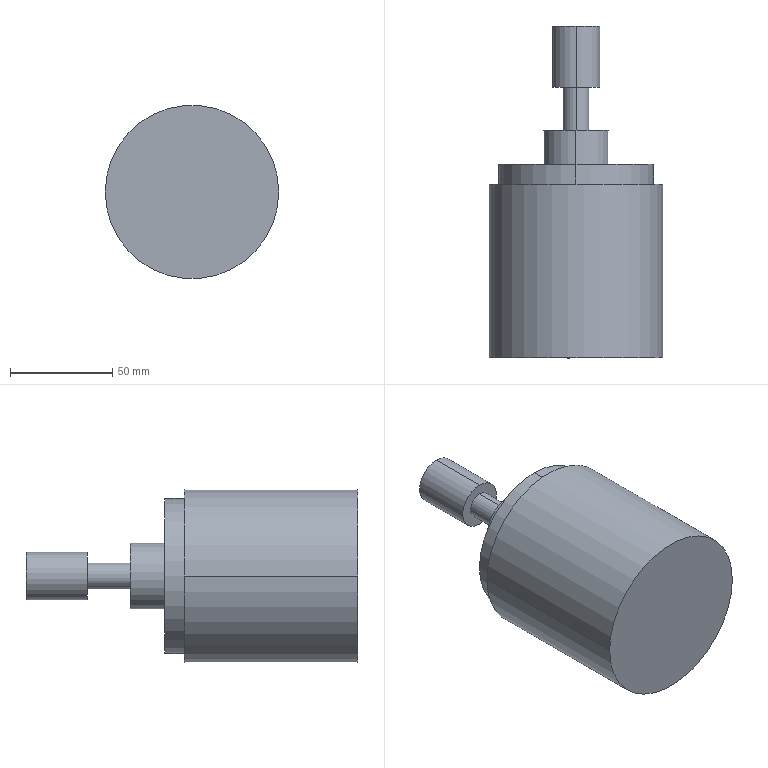Part | SolidWorks | features BaseBody 1 | 1 solid | 22 faces | box 85 x 162.58 x 85 mm | volume 554074 mm3 | cylinder 14 | plane 8 | commonest cylinder face diameters 12.708 x2 23.4 x2 32 x2 34 x2 45 x2 76 x2
STEP:
#1=CARTESIAN_POINT('',(2032.417,122.35,800.897));
#2=VERTEX_POINT('',#1);
#3=CARTESIAN_POINT('',(2032.417,122.35,876.897));
#4=VERTEX_POINT('',#3);
#5=CARTESIAN_POINT('',(2032.417,122.35,838.897));
#6=DIRECTION('',(0.,-1.,0.));
#7=DIRECTION('',(0.,0.,-1.));
#8=AXIS2_PLACEMENT_3D('',#5,#6,#7);
#9=CIRCLE('',#8,38.);
#10=EDGE_CURVE('',#2,#4,#9,.T.);
#11=ORIENTED_EDGE('',*,*,#10,.T.);
#12=CARTESIAN_POINT('',(2032.417,112.6,876.897));
#13=VERTEX_POINT('',#12);
#14=CARTESIAN_POINT('',(2032.417,122.35,876.897));
#15=DIRECTION('',(0.,-1.,0.));
#16=VECTOR('',#15,1000.);
#17=LINE('',#14,#16);
#18=EDGE_CURVE('',#4,#13,#17,.T.);
#19=ORIENTED_EDGE('',*,*,#18,.T.);
#20=CARTESIAN_POINT('',(2032.417,112.6,800.897));
#21=VERTEX_POINT('',#20);
#22=CARTESIAN_POINT('',(2032.417,112.6,838.897));
#23=DIRECTION('',(0.,1.,0.));
#24=DIRECTION('',(0.,0.,-1.));
#25=AXIS2_PLACEMENT_3D('',#22,#23,#24);
#26=CIRCLE('',#25,38.);
#27=EDGE_CURVE('',#13,#21,#26,.T.);
#28=ORIENTED_EDGE('',*,*,#27,.T.);
#29=CARTESIAN_POINT('',(2032.417,122.35,800.897));
#30=DIRECTION('',(0.,-1.,0.));
#31=VECTOR('',#30,1000.);
#32=LINE('',#29,#31);
#33=EDGE_CURVE('',#2,#21,#32,.T.);
#34=ORIENTED_EDGE('',*,*,#33,.F.);
#35=EDGE_LOOP('',(#11,#19,#28,#34));
#36=FACE_OUTER_BOUND('',#35,.T.);
#37=CARTESIAN_POINT('',(2032.417,122.35,838.897));
#38=DIRECTION('',(0.,-1.,0.));
#39=DIRECTION('',(0.,0.,-1.));
#40=AXIS2_PLACEMENT_3D('',#37,#38,#39);
#41=CYLINDRICAL_SURFACE('',#40,38.);
#42=ADVANCED_FACE('',(#36),#41,.T.);
#43=CARTESIAN_POINT('',(2074.917,112.6,838.897));
#44=VERTEX_POINT('',#43);
#45=CARTESIAN_POINT('',(1989.917,112.6,838.897));
#46=VERTEX_POINT('',#45);
#47=CARTESIAN_POINT('',(2032.417,112.6,838.897));
#48=DIRECTION('',(0.,-1.,0.));
#49=DIRECTION('',(0.,0.,1.));
#50=AXIS2_PLACEMENT_3D('',#47,#48,#49);
#51=CIRCLE('',#50,42.5);
#52=EDGE_CURVE('',#44,#46,#51,.T.);
#53=ORIENTED_EDGE('',*,*,#52,.T.);
#54=CARTESIAN_POINT('',(1989.917,27.6,838.897));
#55=VERTEX_POINT('',#54);
#56=CARTESIAN_POINT('',(1989.917,112.6,838.897));
#57=DIRECTION('',(0.,-1.,0.));
#58=VECTOR('',#57,1000.);
#59=LINE('',#56,#58);
#60=EDGE_CURVE('',#46,#55,#59,.T.);
#61=ORIENTED_EDGE('',*,*,#60,.T.);
#62=CARTESIAN_POINT('',(2074.917,27.6,838.897));
#63=VERTEX_POINT('',#62);
#64=CARTESIAN_POINT('',(2032.417,27.6,838.897));
#65=DIRECTION('',(0.,-1.,0.));
#66=DIRECTION('',(0.,0.,1.));
#67=AXIS2_PLACEMENT_3D('',#64,#65,#66);
#68=CIRCLE('',#67,42.5);
#69=EDGE_CURVE('',#63,#55,#68,.T.);
#70=ORIENTED_EDGE('',*,*,#69,.F.);
#71=CARTESIAN_POINT('',(2074.917,112.6,838.897));
#72=DIRECTION('',(0.,-1.,0.));
#73=VECTOR('',#72,1000.);
#74=LINE('',#71,#73);
#75=EDGE_CURVE('',#44,#63,#74,.T.);
#76=ORIENTED_EDGE('',*,*,#75,.F.);
#77=EDGE_LOOP('',(#53,#61,#70,#76));
#78=FACE_OUTER_BOUND('',#77,.T.);
#79=CARTESIAN_POINT('',(2032.417,112.6,838.897));
#80=DIRECTION('',(0.,-1.,0.));
#81=DIRECTION('',(1.,0.,0.));
#82=AXIS2_PLACEMENT_3D('',#79,#80,#81);
#83=CYLINDRICAL_SURFACE('',#82,42.5);
#84=ADVANCED_FACE('',(#78),#83,.T.);
#85=CARTESIAN_POINT('',(2032.457,122.35,861.389));
#86=VERTEX_POINT('',#85);
#87=CARTESIAN_POINT('',(2032.457,122.35,816.389));
#88=VERTEX_POINT('',#87);
#89=CARTESIAN_POINT('',(2032.457,122.35,838.889));
#90=DIRECTION('',(0.,-1.,0.));
#91=DIRECTION('',(0.,0.,-1.));
#92=AXIS2_PLACEMENT_3D('',#89,#90,#91);
#93=CIRCLE('',#92,22.5);
#94=EDGE_CURVE('',#86,#88,#93,.T.);
#95=ORIENTED_EDGE('',*,*,#94,.F.);
#96=CARTESIAN_POINT('',(2032.457,120.1,861.389));
#97=VERTEX_POINT('',#96);
#98=CARTESIAN_POINT('',(2032.457,130.6,861.389));
#99=DIRECTION('',(0.,-1.,0.));
#100=VECTOR('',#99,1000.);
#101=LINE('',#98,#100);
#102=EDGE_CURVE('',#86,#97,#101,.T.);
#103=ORIENTED_EDGE('',*,*,#102,.T.);
#104=CARTESIAN_POINT('',(2032.457,120.1,816.389));
#105=VERTEX_POINT('',#104);
#106=CARTESIAN_POINT('',(2032.457,120.1,838.889));
#107=DIRECTION('',(0.,-1.,0.));
#108=DIRECTION('',(-0.84,0.,-0.5427));
#109=AXIS2_PLACEMENT_3D('',#106,#107,#108);
#110=CIRCLE('',#109,22.5);
#111=EDGE_CURVE('',#97,#105,#110,.T.);
#112=ORIENTED_EDGE('',*,*,#111,.T.);
#113=CARTESIAN_POINT('',(2032.457,130.6,816.389));
#114=DIRECTION('',(0.,-1.,0.));
#115=VECTOR('',#114,1000.);
#116=LINE('',#113,#115);
#117=EDGE_CURVE('',#88,#105,#116,.T.);
#118=ORIENTED_EDGE('',*,*,#117,.F.);
#119=EDGE_LOOP('',(#95,#103,#112,#118));
#120=FACE_OUTER_BOUND('',#119,.T.);
#121=CARTESIAN_POINT('',(2032.457,130.6,838.889));
#122=DIRECTION('',(0.,-1.,0.));
#123=DIRECTION('',(0.,0.,-1.));
#124=AXIS2_PLACEMENT_3D('',#121,#122,#123);
#125=CYLINDRICAL_SURFACE('',#124,22.5);
#126=ADVANCED_FACE('',(#120),#125,.F.);
#127=CARTESIAN_POINT('',(2032.457,120.1,821.889));
#128=VERTEX_POINT('',#127);
#129=CARTESIAN_POINT('',(2032.457,120.1,855.889));
#130=VERTEX_POINT('',#129);
#131=CARTESIAN_POINT('',(2032.457,120.1,838.889));
#132=DIRECTION('',(0.,-1.,0.));
#133=DIRECTION('',(-0.9306,0.,-0.366));
#134=AXIS2_PLACEMENT_3D('',#131,#132,#133);
#135=CIRCLE('',#134,17.);
#136=EDGE_CURVE('',#128,#130,#135,.T.);
#137=ORIENTED_EDGE('',*,*,#136,.F.);
#138=CARTESIAN_POINT('',(2032.457,122.35,821.889));
#139=VERTEX_POINT('',#138);
#140=CARTESIAN_POINT('',(2032.457,120.1,821.889));
#141=DIRECTION('',(0.,1.,0.));
#142=VECTOR('',#141,1000.);
#143=LINE('',#140,#142);
#144=EDGE_CURVE('',#128,#139,#143,.T.);
#145=ORIENTED_EDGE('',*,*,#144,.T.);
#146=CARTESIAN_POINT('',(2032.457,122.35,855.889));
#147=VERTEX_POINT('',#146);
#148=CARTESIAN_POINT('',(2032.457,122.35,838.889));
#149=DIRECTION('',(0.,-1.,0.));
#150=DIRECTION('',(0.,0.,-1.));
#151=AXIS2_PLACEMENT_3D('',#148,#149,#150);
#152=CIRCLE('',#151,17.);
#153=EDGE_CURVE('',#139,#147,#152,.T.);
#154=ORIENTED_EDGE('',*,*,#153,.T.);
#155=CARTESIAN_POINT('',(2032.457,120.1,855.889));
#156=DIRECTION('',(0.,1.,0.));
#157=VECTOR('',#156,1000.);
#158=LINE('',#155,#157);
#159=EDGE_CURVE('',#130,#147,#158,.T.);
#160=ORIENTED_EDGE('',*,*,#159,.F.);
#161=EDGE_LOOP('',(#137,#145,#154,#160));
#162=FACE_OUTER_BOUND('',#161,.T.);
#163=CARTESIAN_POINT('',(2032.457,120.1,838.889));
#164=DIRECTION('',(0.,1.,0.));
#165=DIRECTION('',(0.,0.,1.));
#166=AXIS2_PLACEMENT_3D('',#163,#164,#165);
#167=CYLINDRICAL_SURFACE('',#166,17.);
#168=ADVANCED_FACE('',(#162),#167,.T.);
#169=CARTESIAN_POINT('',(2032.457,190.18,850.589));
#170=VERTEX_POINT('',#169);
#171=CARTESIAN_POINT('',(2032.457,190.18,827.189));
#172=VERTEX_POINT('',#171);
#173=CARTESIAN_POINT('',(2032.457,190.18,838.889));
#174=DIRECTION('',(0.,1.,0.));
#175=DIRECTION('',(-0.1749,0.,-0.9846));
#176=AXIS2_PLACEMENT_3D('',#173,#174,#175);
#177=CIRCLE('',#176,11.7);
#178=EDGE_CURVE('',#170,#172,#177,.T.);
#179=ORIENTED_EDGE('',*,*,#178,.F.);
#180=CARTESIAN_POINT('',(2032.457,160.18,850.589));
#181=VERTEX_POINT('',#180);
#182=CARTESIAN_POINT('',(2032.457,190.18,850.589));
#183=DIRECTION('',(0.,-1.,0.));
#184=VECTOR('',#183,1000.);
#185=LINE('',#182,#184);
#186=EDGE_CURVE('',#170,#181,#185,.T.);
#187=ORIENTED_EDGE('',*,*,#186,.T.);
#188=CARTESIAN_POINT('',(2032.457,160.18,827.189));
#189=VERTEX_POINT('',#188);
#190=CARTESIAN_POINT('',(2032.457,160.18,838.889));
#191=DIRECTION('',(0.,1.,0.));
#192=DIRECTION('',(0.1749,0.,0.9846));
#193=AXIS2_PLACEMENT_3D('',#190,#191,#192);
#194=CIRCLE('',#193,11.7);
#195=EDGE_CURVE('',#181,#189,#194,.T.);
#196=ORIENTED_EDGE('',*,*,#195,.T.);
#197=CARTESIAN_POINT('',(2032.457,190.18,827.189));
#198=DIRECTION('',(0.,-1.,0.));
#199=VECTOR('',#198,1000.);
#200=LINE('',#197,#199);
#201=EDGE_CURVE('',#172,#189,#200,.T.);
#202=ORIENTED_EDGE('',*,*,#201,.F.);
#203=EDGE_LOOP('',(#179,#187,#196,#202));
#204=FACE_OUTER_BOUND('',#203,.T.);
#205=CARTESIAN_POINT('',(2032.457,190.18,838.889));
#206=DIRECTION('',(0.,-1.,0.));
#207=DIRECTION('',(0.,0.,-1.));
#208=AXIS2_PLACEMENT_3D('',#205,#206,#207);
#209=CYLINDRICAL_SURFACE('',#208,11.7);
#210=ADVANCED_FACE('',(#204),#209,.T.);
#211=CARTESIAN_POINT('',(2032.457,160.18,845.243));
#212=VERTEX_POINT('',#211);
#213=CARTESIAN_POINT('',(2032.457,160.18,832.535));
#214=VERTEX_POINT('',#213);
#215=CARTESIAN_POINT('',(2032.457,160.18,838.889));
#216=DIRECTION('',(0.,1.,0.));
#217=DIRECTION('',(0.,0.,1.));
#218=AXIS2_PLACEMENT_3D('',#215,#216,#217);
#219=CIRCLE('',#218,6.354);
#220=EDGE_CURVE('',#212,#214,#219,.T.);
#221=ORIENTED_EDGE('',*,*,#220,.F.);
#222=CARTESIAN_POINT('',(2032.457,139.1,845.243));
#223=VERTEX_POINT('',#222);
#224=CARTESIAN_POINT('',(2032.457,162.7,845.243));
#225=DIRECTION('',(0.,-1.,0.));
#226=VECTOR('',#225,1000.);
#227=LINE('',#224,#226);
#228=EDGE_CURVE('',#212,#223,#227,.T.);
#229=ORIENTED_EDGE('',*,*,#228,.T.);
#230=CARTESIAN_POINT('',(2032.457,139.1,832.535));
#231=VERTEX_POINT('',#230);
#232=CARTESIAN_POINT('',(2032.457,139.1,838.889));
#233=DIRECTION('',(0.,1.,0.));
#234=DIRECTION('',(1.,0.,0.));
#235=AXIS2_PLACEMENT_3D('',#232,#233,#234);
#236=CIRCLE('',#235,6.354);
#237=EDGE_CURVE('',#223,#231,#236,.T.);
#238=ORIENTED_EDGE('',*,*,#237,.T.);
#239=CARTESIAN_POINT('',(2032.457,162.7,832.535));
#240=DIRECTION('',(0.,-1.,0.));
#241=VECTOR('',#240,1000.);
#242=LINE('',#239,#241);
#243=EDGE_CURVE('',#214,#231,#242,.T.);
#244=ORIENTED_EDGE('',*,*,#243,.F.);
#245=EDGE_LOOP('',(#221,#229,#238,#244));
#246=FACE_OUTER_BOUND('',#245,.T.);
#247=CARTESIAN_POINT('',(2032.457,162.7,838.889));
#248=DIRECTION('',(0.,-1.,0.));
#249=DIRECTION('',(0.,0.,-1.));
#250=AXIS2_PLACEMENT_3D('',#247,#248,#249);
#251=CYLINDRICAL_SURFACE('',#250,6.354);
#252=ADVANCED_FACE('',(#246),#251,.T.);
#253=CARTESIAN_POINT('',(2032.417,139.1,822.897));
#254=VERTEX_POINT('',#253);
#255=CARTESIAN_POINT('',(2032.417,139.1,854.897));
#256=VERTEX_POINT('',#255);
#257=CARTESIAN_POINT('',(2032.417,139.1,838.897));
#258=DIRECTION('',(0.,-1.,0.));
#259=DIRECTION('',(0.,0.,1.));
#260=AXIS2_PLACEMENT_3D('',#257,#258,#259);
#261=CIRCLE('',#260,16.);
#262=EDGE_CURVE('',#254,#256,#261,.T.);
#263=ORIENTED_EDGE('',*,*,#262,.T.);
#264=CARTESIAN_POINT('',(2032.417,122.35,854.897));
#265=VERTEX_POINT('',#264);
#266=CARTESIAN_POINT('',(2032.417,139.1,854.897));
#267=DIRECTION('',(0.,-1.,0.));
#268=VECTOR('',#267,1000.);
#269=LINE('',#266,#268);
#270=EDGE_CURVE('',#256,#265,#269,.T.);
#271=ORIENTED_EDGE('',*,*,#270,.T.);
#272=CARTESIAN_POINT('',(2032.417,122.35,822.897));
#273=VERTEX_POINT('',#272);
#274=CARTESIAN_POINT('',(2032.417,122.35,838.897));
#275=DIRECTION('',(0.,-1.,0.));
#276=DIRECTION('',(0.,0.,-1.));
#277=AXIS2_PLACEMENT_3D('',#274,#275,#276);
#278=CIRCLE('',#277,16.);
#279=EDGE_CURVE('',#273,#265,#278,.T.);
#280=ORIENTED_EDGE('',*,*,#279,.F.);
#281=CARTESIAN_POINT('',(2032.417,139.1,822.897));
#282=DIRECTION('',(0.,-1.,0.));
#283=VECTOR('',#282,1000.);
#284=LINE('',#281,#283);
#285=EDGE_CURVE('',#254,#273,#284,.T.);
#286=ORIENTED_EDGE('',*,*,#285,.F.);
#287=EDGE_LOOP('',(#263,#271,#280,#286));
#288=FACE_OUTER_BOUND('',#287,.T.);
#289=CARTESIAN_POINT('',(2032.417,139.1,838.897));
#290=DIRECTION('',(0.,-1.,0.));
#291=DIRECTION('',(0.,0.,-1.));
#292=AXIS2_PLACEMENT_3D('',#289,#290,#291);
#293=CYLINDRICAL_SURFACE('',#292,16.);
#294=ADVANCED_FACE('',(#288),#293,.T.);
#295=ORIENTED_EDGE('',*,*,#279,.T.);
#296=CARTESIAN_POINT('',(2032.417,122.35,838.897));
#297=DIRECTION('',(0.,-1.,0.));
#298=DIRECTION('',(0.,0.,-1.));
#299=AXIS2_PLACEMENT_3D('',#296,#297,#298);
#300=CIRCLE('',#299,16.);
#301=EDGE_CURVE('',#265,#273,#300,.T.);
#302=ORIENTED_EDGE('',*,*,#301,.T.);
#303=EDGE_LOOP('',(#295,#302));
#304=FACE_BOUND('',#303,.T.);
#305=CARTESIAN_POINT('',(2032.457,122.35,838.889));
#306=DIRECTION('',(0.,-1.,0.));
#307=DIRECTION('',(0.,0.,-1.));
#308=AXIS2_PLACEMENT_3D('',#305,#306,#307);
#309=CIRCLE('',#308,17.);
#310=EDGE_CURVE('',#147,#139,#309,.T.);
#311=ORIENTED_EDGE('',*,*,#310,.F.);
#312=ORIENTED_EDGE('',*,*,#153,.F.);
#313=EDGE_LOOP('',(#311,#312));
#314=FACE_OUTER_BOUND('',#313,.T.);
#315=CARTESIAN_POINT('',(2032.417,122.35,838.897));
#316=DIRECTION('',(0.,-1.,0.));
#317=DIRECTION('',(0.,0.,-1.));
#318=AXIS2_PLACEMENT_3D('',#315,#316,#317);
#319=PLANE('',#318);
#320=ADVANCED_FACE('',(#304,#314),#319,.F.);
#321=ORIENTED_EDGE('',*,*,#270,.F.);
#322=CARTESIAN_POINT('',(2032.417,139.1,838.897));
#323=DIRECTION('',(0.,-1.,0.));
#324=DIRECTION('',(0.,0.,1.));
#325=AXIS2_PLACEMENT_3D('',#322,#323,#324);
#326=CIRCLE('',#325,16.);
#327=EDGE_CURVE('',#256,#254,#326,.T.);
#328=ORIENTED_EDGE('',*,*,#327,.T.);
#329=ORIENTED_EDGE('',*,*,#285,.T.);
#330=ORIENTED_EDGE('',*,*,#301,.F.);
#331=EDGE_LOOP('',(#321,#328,#329,#330));
#332=FACE_OUTER_BOUND('',#331,.T.);
#333=CARTESIAN_POINT('',(2032.417,139.1,838.897));
#334=DIRECTION('',(0.,-1.,0.));
#335=DIRECTION('',(0.,0.,-1.));
#336=AXIS2_PLACEMENT_3D('',#333,#334,#335);
#337=CYLINDRICAL_SURFACE('',#336,16.);
#338=ADVANCED_FACE('',(#332),#337,.T.);
#339=ORIENTED_EDGE('',*,*,#228,.F.);
#340=CARTESIAN_POINT('',(2032.457,160.18,838.889));
#341=DIRECTION('',(0.,1.,0.));
#342=DIRECTION('',(0.,0.,1.));
#343=AXIS2_PLACEMENT_3D('',#340,#341,#342);
#344=CIRCLE('',#343,6.354);
#345=EDGE_CURVE('',#214,#212,#344,.T.);
#346=ORIENTED_EDGE('',*,*,#345,.F.);
#347=ORIENTED_EDGE('',*,*,#243,.T.);
#348=CARTESIAN_POINT('',(2032.457,139.1,838.889));
#349=DIRECTION('',(0.,1.,0.));
#350=DIRECTION('',(1.,0.,0.));
#351=AXIS2_PLACEMENT_3D('',#348,#349,#350);
#352=CIRCLE('',#351,6.354);
#353=EDGE_CURVE('',#231,#223,#352,.T.);
#354=ORIENTED_EDGE('',*,*,#353,.T.);
#355=EDGE_LOOP('',(#339,#346,#347,#354));
#356=FACE_OUTER_BOUND('',#355,.T.);
#357=CARTESIAN_POINT('',(2032.457,162.7,838.889));
#358=DIRECTION('',(0.,-1.,0.));
#359=DIRECTION('',(0.,0.,-1.));
#360=AXIS2_PLACEMENT_3D('',#357,#358,#359);
#361=CYLINDRICAL_SURFACE('',#360,6.354);
#362=ADVANCED_FACE('',(#356),#361,.T.);
#363=ORIENTED_EDGE('',*,*,#186,.F.);
#364=CARTESIAN_POINT('',(2032.457,190.18,838.889));
#365=DIRECTION('',(0.,1.,0.));
#366=DIRECTION('',(-0.1749,0.,-0.9846));
#367=AXIS2_PLACEMENT_3D('',#364,#365,#366);
#368=CIRCLE('',#367,11.7);
#369=EDGE_CURVE('',#172,#170,#368,.T.);
#370=ORIENTED_EDGE('',*,*,#369,.F.);
#371=ORIENTED_EDGE('',*,*,#201,.T.);
#372=CARTESIAN_POINT('',(2032.457,160.18,838.889));
#373=DIRECTION('',(0.,1.,0.));
#374=DIRECTION('',(0.1749,0.,0.9846));
#375=AXIS2_PLACEMENT_3D('',#372,#373,#374);
#376=CIRCLE('',#375,11.7);
#377=EDGE_CURVE('',#189,#181,#376,.T.);
#378=ORIENTED_EDGE('',*,*,#377,.T.);
#379=EDGE_LOOP('',(#363,#370,#371,#378));
#380=FACE_OUTER_BOUND('',#379,.T.);
#381=CARTESIAN_POINT('',(2032.457,190.18,838.889));
#382=DIRECTION('',(0.,-1.,0.));
#383=DIRECTION('',(0.,0.,-1.));
#384=AXIS2_PLACEMENT_3D('',#381,#382,#383);
#385=CYLINDRICAL_SURFACE('',#384,11.7);
#386=ADVANCED_FACE('',(#380),#385,.T.);
#387=ORIENTED_EDGE('',*,*,#369,.T.);
#388=ORIENTED_EDGE('',*,*,#178,.T.);
#389=EDGE_LOOP('',(#387,#388));
#390=FACE_OUTER_BOUND('',#389,.T.);
#391=CARTESIAN_POINT('',(2032.457,190.18,838.889));
#392=DIRECTION('',(0.,1.,0.));
#393=DIRECTION('',(0.,0.,1.));
#394=AXIS2_PLACEMENT_3D('',#391,#392,#393);
#395=PLANE('',#394);
#396=ADVANCED_FACE('',(#390),#395,.T.);
#397=ORIENTED_EDGE('',*,*,#345,.T.);
#398=ORIENTED_EDGE('',*,*,#220,.T.);
#399=EDGE_LOOP('',(#397,#398));
#400=FACE_BOUND('',#399,.T.);
#401=ORIENTED_EDGE('',*,*,#377,.F.);
#402=ORIENTED_EDGE('',*,*,#195,.F.);
#403=EDGE_LOOP('',(#401,#402));
#404=FACE_OUTER_BOUND('',#403,.T.);
#405=CARTESIAN_POINT('',(2032.457,160.18,838.889));
#406=DIRECTION('',(0.,1.,0.));
#407=DIRECTION('',(0.,0.,1.));
#408=AXIS2_PLACEMENT_3D('',#405,#406,#407);
#409=PLANE('',#408);
#410=ADVANCED_FACE('',(#400,#404),#409,.F.);
#411=ORIENTED_EDGE('',*,*,#353,.F.);
#412=ORIENTED_EDGE('',*,*,#237,.F.);
#413=EDGE_LOOP('',(#411,#412));
#414=FACE_BOUND('',#413,.T.);
#415=ORIENTED_EDGE('',*,*,#262,.F.);
#416=ORIENTED_EDGE('',*,*,#327,.F.);
#417=EDGE_LOOP('',(#415,#416));
#418=FACE_OUTER_BOUND('',#417,.T.);
#419=CARTESIAN_POINT('',(2032.417,139.1,838.897));
#420=DIRECTION('',(0.,-1.,0.));
#421=DIRECTION('',(1.,0.,0.));
#422=AXIS2_PLACEMENT_3D('',#419,#420,#421);
#423=PLANE('',#422);
#424=ADVANCED_FACE('',(#414,#418),#423,.F.);
#425=ORIENTED_EDGE('',*,*,#144,.F.);
#426=CARTESIAN_POINT('',(2032.457,120.1,838.889));
#427=DIRECTION('',(0.,-1.,0.));
#428=DIRECTION('',(-0.9306,0.,-0.366));
#429=AXIS2_PLACEMENT_3D('',#426,#427,#428);
#430=CIRCLE('',#429,17.);
#431=EDGE_CURVE('',#130,#128,#430,.T.);
#432=ORIENTED_EDGE('',*,*,#431,.F.);
#433=ORIENTED_EDGE('',*,*,#159,.T.);
#434=ORIENTED_EDGE('',*,*,#310,.T.);
#435=EDGE_LOOP('',(#425,#432,#433,#434));
#436=FACE_OUTER_BOUND('',#435,.T.);
#437=CARTESIAN_POINT('',(2032.457,120.1,838.889));
#438=DIRECTION('',(0.,1.,0.));
#439=DIRECTION('',(0.,0.,1.));
#440=AXIS2_PLACEMENT_3D('',#437,#438,#439);
#441=CYLINDRICAL_SURFACE('',#440,17.);
#442=ADVANCED_FACE('',(#436),#441,.T.);
#443=ORIENTED_EDGE('',*,*,#431,.T.);
#444=ORIENTED_EDGE('',*,*,#136,.T.);
#445=EDGE_LOOP('',(#443,#444));
#446=FACE_BOUND('',#445,.T.);
#447=CARTESIAN_POINT('',(2032.457,120.1,838.889));
#448=DIRECTION('',(0.,-1.,0.));
#449=DIRECTION('',(-0.84,0.,-0.5427));
#450=AXIS2_PLACEMENT_3D('',#447,#448,#449);
#451=CIRCLE('',#450,22.5);
#452=EDGE_CURVE('',#105,#97,#451,.T.);
#453=ORIENTED_EDGE('',*,*,#452,.F.);
#454=ORIENTED_EDGE('',*,*,#111,.F.);
#455=EDGE_LOOP('',(#453,#454));
#456=FACE_OUTER_BOUND('',#455,.T.);
#457=CARTESIAN_POINT('',(2032.457,120.1,838.889));
#458=DIRECTION('',(0.,1.,0.));
#459=DIRECTION('',(0.,0.,1.));
#460=AXIS2_PLACEMENT_3D('',#457,#458,#459);
#461=PLANE('',#460);
#462=ADVANCED_FACE('',(#446,#456),#461,.T.);
#463=ORIENTED_EDGE('',*,*,#102,.F.);
#464=CARTESIAN_POINT('',(2032.457,122.35,838.889));
#465=DIRECTION('',(0.,-1.,0.));
#466=DIRECTION('',(0.,0.,-1.));
#467=AXIS2_PLACEMENT_3D('',#464,#465,#466);
#468=CIRCLE('',#467,22.5);
#469=EDGE_CURVE('',#88,#86,#468,.T.);
#470=ORIENTED_EDGE('',*,*,#469,.F.);
#471=ORIENTED_EDGE('',*,*,#117,.T.);
#472=ORIENTED_EDGE('',*,*,#452,.T.);
#473=EDGE_LOOP('',(#463,#470,#471,#472));
#474=FACE_OUTER_BOUND('',#473,.T.);
#475=CARTESIAN_POINT('',(2032.457,130.6,838.889));
#476=DIRECTION('',(0.,-1.,0.));
#477=DIRECTION('',(0.,0.,-1.));
#478=AXIS2_PLACEMENT_3D('',#475,#476,#477);
#479=CYLINDRICAL_SURFACE('',#478,22.5);
#480=ADVANCED_FACE('',(#474),#479,.F.);
#481=ORIENTED_EDGE('',*,*,#69,.T.);
#482=CARTESIAN_POINT('',(2032.417,27.6,838.897));
#483=DIRECTION('',(0.,-1.,0.));
#484=DIRECTION('',(0.,0.,1.));
#485=AXIS2_PLACEMENT_3D('',#482,#483,#484);
#486=CIRCLE('',#485,42.5);
#487=EDGE_CURVE('',#55,#63,#486,.T.);
#488=ORIENTED_EDGE('',*,*,#487,.T.);
#489=EDGE_LOOP('',(#481,#488));
#490=FACE_OUTER_BOUND('',#489,.T.);
#491=CARTESIAN_POINT('',(2032.417,27.6,838.897));
#492=DIRECTION('',(0.,-1.,0.));
#493=DIRECTION('',(1.,0.,0.));
#494=AXIS2_PLACEMENT_3D('',#491,#492,#493);
#495=PLANE('',#494);
#496=ADVANCED_FACE('',(#490),#495,.T.);
#497=ORIENTED_EDGE('',*,*,#60,.F.);
#498=CARTESIAN_POINT('',(2032.417,112.6,838.897));
#499=DIRECTION('',(0.,-1.,0.));
#500=DIRECTION('',(0.,0.,1.));
#501=AXIS2_PLACEMENT_3D('',#498,#499,#500);
#502=CIRCLE('',#501,42.5);
#503=EDGE_CURVE('',#46,#44,#502,.T.);
#504=ORIENTED_EDGE('',*,*,#503,.T.);
#505=ORIENTED_EDGE('',*,*,#75,.T.);
#506=ORIENTED_EDGE('',*,*,#487,.F.);
#507=EDGE_LOOP('',(#497,#504,#505,#506));
#508=FACE_OUTER_BOUND('',#507,.T.);
#509=CARTESIAN_POINT('',(2032.417,112.6,838.897));
#510=DIRECTION('',(0.,-1.,0.));
#511=DIRECTION('',(1.,0.,0.));
#512=AXIS2_PLACEMENT_3D('',#509,#510,#511);
#513=CYLINDRICAL_SURFACE('',#512,42.5);
#514=ADVANCED_FACE('',(#508),#513,.T.);
#515=CARTESIAN_POINT('',(2032.417,112.6,838.897));
#516=DIRECTION('',(0.,1.,0.));
#517=DIRECTION('',(0.,0.,-1.));
#518=AXIS2_PLACEMENT_3D('',#515,#516,#517);
#519=CIRCLE('',#518,38.);
#520=EDGE_CURVE('',#21,#13,#519,.T.);
#521=ORIENTED_EDGE('',*,*,#520,.F.);
#522=ORIENTED_EDGE('',*,*,#27,.F.);
#523=EDGE_LOOP('',(#521,#522));
#524=FACE_BOUND('',#523,.T.);
#525=ORIENTED_EDGE('',*,*,#52,.F.);
#526=ORIENTED_EDGE('',*,*,#503,.F.);
#527=EDGE_LOOP('',(#525,#526));
#528=FACE_OUTER_BOUND('',#527,.T.);
#529=CARTESIAN_POINT('',(2032.417,112.6,838.897));
#530=DIRECTION('',(0.,-1.,0.));
#531=DIRECTION('',(1.,0.,0.));
#532=AXIS2_PLACEMENT_3D('',#529,#530,#531);
#533=PLANE('',#532);
#534=ADVANCED_FACE('',(#524,#528),#533,.F.);
#535=ORIENTED_EDGE('',*,*,#18,.F.);
#536=CARTESIAN_POINT('',(2032.417,122.35,838.897));
#537=DIRECTION('',(0.,-1.,0.));
#538=DIRECTION('',(0.,0.,-1.));
#539=AXIS2_PLACEMENT_3D('',#536,#537,#538);
#540=CIRCLE('',#539,38.);
#541=EDGE_CURVE('',#4,#2,#540,.T.);
#542=ORIENTED_EDGE('',*,*,#541,.T.);
#543=ORIENTED_EDGE('',*,*,#33,.T.);
#544=ORIENTED_EDGE('',*,*,#520,.T.);
#545=EDGE_LOOP('',(#535,#542,#543,#544));
#546=FACE_OUTER_BOUND('',#545,.T.);
#547=CARTESIAN_POINT('',(2032.417,122.35,838.897));
#548=DIRECTION('',(0.,-1.,0.));
#549=DIRECTION('',(0.,0.,-1.));
#550=AXIS2_PLACEMENT_3D('',#547,#548,#549);
#551=CYLINDRICAL_SURFACE('',#550,38.);
#552=ADVANCED_FACE('',(#546),#551,.T.);
#553=ORIENTED_EDGE('',*,*,#469,.T.);
#554=ORIENTED_EDGE('',*,*,#94,.T.);
#555=EDGE_LOOP('',(#553,#554));
#556=FACE_BOUND('',#555,.T.);
#557=ORIENTED_EDGE('',*,*,#10,.F.);
#558=ORIENTED_EDGE('',*,*,#541,.F.);
#559=EDGE_LOOP('',(#557,#558));
#560=FACE_OUTER_BOUND('',#559,.T.);
#561=CARTESIAN_POINT('',(2032.417,122.35,838.897));
#562=DIRECTION('',(0.,-1.,0.));
#563=DIRECTION('',(0.,0.,-1.));
#564=AXIS2_PLACEMENT_3D('',#561,#562,#563);
#565=PLANE('',#564);
#566=ADVANCED_FACE('',(#556,#560),#565,.F.);
#567=CLOSED_SHELL('',(#42,#84,#126,#168,#210,#252,#294,#320,#338,#362,#386,#396,#410,#424,#442,#462,#480,#496,#514,#534,#552,#566));
#568=MANIFOLD_SOLID_BREP('',#567);
#569=CARTESIAN_POINT('',(0.,0.,0.));
#570=DIRECTION('',(0.,0.,1.));
#571=DIRECTION('',(1.,0.,0.));
#572=AXIS2_PLACEMENT_3D('',#569,#570,#571);
#573=(LENGTH_UNIT()NAMED_UNIT(*)SI_UNIT(.MILLI.,.METRE.));
#574=UNCERTAINTY_MEASURE_WITH_UNIT(LENGTH_MEASURE(0.00001),#573,'','');
#575=(NAMED_UNIT(*)PLANE_ANGLE_UNIT()SI_UNIT($,.RADIAN.));
#576=(NAMED_UNIT(*)SI_UNIT($,.STERADIAN.)SOLID_ANGLE_UNIT());
#577=(GEOMETRIC_REPRESENTATION_CONTEXT(3)GLOBAL_UNCERTAINTY_ASSIGNED_CONTEXT((#574))GLOBAL_UNIT_ASSIGNED_CONTEXT((#573,#575,#576))REPRESENTATION_CONTEXT('',''));
#578=ADVANCED_BREP_SHAPE_REPRESENTATION('',(#568,#572),#577);